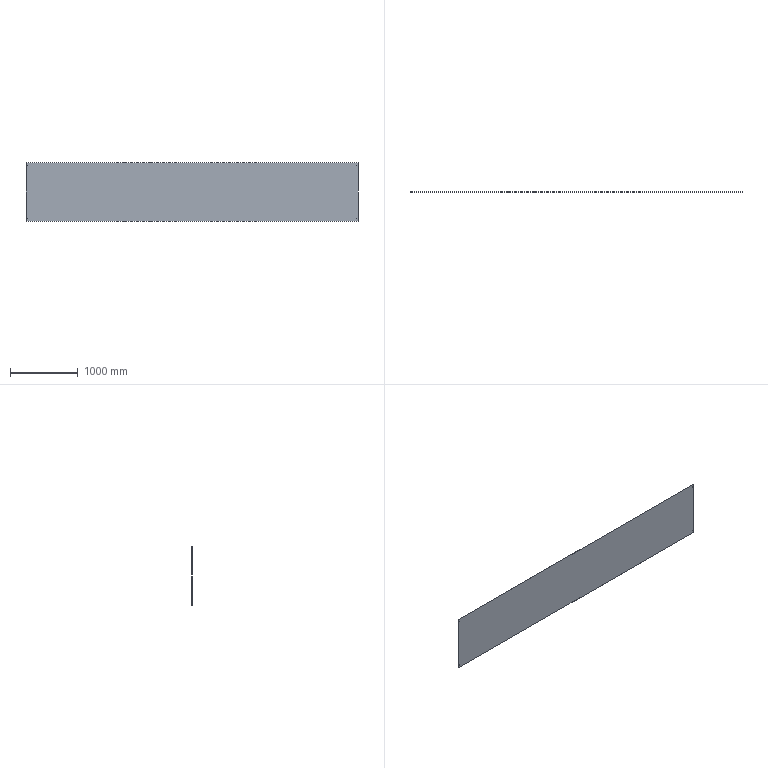Part | STEP file | 01-Cover plate | 1 solid | 14 faces | box 4900 x 0.6 x 870 mm | volume 2557612 mm3 | cylinder 8 | plane 6 | commonest cylinder face diameters 10 x8
STEP:
#1=CARTESIAN_POINT('',(0.,0.,0.));
#2=DIRECTION('',(0.,0.,1.));
#3=DIRECTION('',(1.,0.,0.));
#4=AXIS2_PLACEMENT_3D('',#1,#2,#3);
#5=CARTESIAN_POINT('',(4880.,0.,830.));
#6=VERTEX_POINT('',#5);
#7=CARTESIAN_POINT('',(4880.,0.6,830.));
#8=VERTEX_POINT('',#7);
#9=CARTESIAN_POINT('',(4880.,-19.4,830.));
#10=DIRECTION('',(0.,1.,0.));
#11=VECTOR('',#10,1.);
#12=LINE('',#9,#11);
#13=CARTESIAN_POINT('',(4880.,-19.4,825.));
#14=DIRECTION('',(0.,1.,0.));
#15=DIRECTION('',(0.,0.,1.));
#16=AXIS2_PLACEMENT_3D('',#13,#14,#15);
#17=CYLINDRICAL_SURFACE('',#16,5.);
#18=CARTESIAN_POINT('',(6.283,0.));
#19=DIRECTION('',(0.,1.));
#20=VECTOR('',#19,1.);
#21=LINE('',#18,#20);
#22=(GEOMETRIC_REPRESENTATION_CONTEXT(2)PARAMETRIC_REPRESENTATION_CONTEXT()REPRESENTATION_CONTEXT('',''));
#23=DEFINITIONAL_REPRESENTATION('',(#21),#22);
#24=PCURVE('',#17,#23);
#25=CARTESIAN_POINT('',(4880.,-19.4,825.));
#26=DIRECTION('',(0.,1.,0.));
#27=DIRECTION('',(0.,0.,1.));
#28=AXIS2_PLACEMENT_3D('',#25,#26,#27);
#29=CYLINDRICAL_SURFACE('',#28,5.);
#30=CARTESIAN_POINT('',(0.,0.));
#31=DIRECTION('',(0.,1.));
#32=VECTOR('',#31,1.);
#33=LINE('',#30,#32);
#34=(GEOMETRIC_REPRESENTATION_CONTEXT(2)PARAMETRIC_REPRESENTATION_CONTEXT()REPRESENTATION_CONTEXT('',''));
#35=DEFINITIONAL_REPRESENTATION('',(#33),#34);
#36=PCURVE('',#29,#35);
#37=SURFACE_CURVE('',#12,(#24,#36),.PCURVE_S1.);
#38=EDGE_CURVE('',#6,#8,#37,.T.);
#39=ORIENTED_EDGE('',*,*,#38,.T.);
#40=CARTESIAN_POINT('',(4880.,0.6,820.));
#41=VERTEX_POINT('',#40);
#42=CARTESIAN_POINT('',(4880.,0.6,825.));
#43=DIRECTION('',(0.,1.,0.));
#44=DIRECTION('',(0.,0.,1.));
#45=AXIS2_PLACEMENT_3D('',#42,#43,#44);
#46=CIRCLE('',#45,5.);
#47=CARTESIAN_POINT('',(0.,20.));
#48=DIRECTION('',(1.,0.));
#49=VECTOR('',#48,1.);
#50=LINE('',#47,#49);
#51=(GEOMETRIC_REPRESENTATION_CONTEXT(2)PARAMETRIC_REPRESENTATION_CONTEXT()REPRESENTATION_CONTEXT('',''));
#52=DEFINITIONAL_REPRESENTATION('',(#50),#51);
#53=PCURVE('',#17,#52);
#54=CARTESIAN_POINT('',(0.,0.6,0.));
#55=DIRECTION('',(0.,1.,0.));
#56=DIRECTION('',(0.,0.,1.));
#57=AXIS2_PLACEMENT_3D('',#54,#55,#56);
#58=PLANE('',#57);
#59=CARTESIAN_POINT('',(825.,4880.));
#60=DIRECTION('',(1.,0.));
#61=AXIS2_PLACEMENT_2D('',#59,#60);
#62=CIRCLE('',#61,5.);
#63=(GEOMETRIC_REPRESENTATION_CONTEXT(2)PARAMETRIC_REPRESENTATION_CONTEXT()REPRESENTATION_CONTEXT('',''));
#64=DEFINITIONAL_REPRESENTATION('',(#62),#63);
#65=PCURVE('',#58,#64);
#66=SURFACE_CURVE('',#46,(#53,#65),.PCURVE_S1.);
#67=EDGE_CURVE('',#41,#8,#66,.T.);
#68=ORIENTED_EDGE('',*,*,#67,.F.);
#69=CARTESIAN_POINT('',(4880.,0.,820.));
#70=VERTEX_POINT('',#69);
#71=CARTESIAN_POINT('',(4880.,-19.4,820.));
#72=DIRECTION('',(0.,1.,0.));
#73=VECTOR('',#72,1.);
#74=LINE('',#71,#73);
#75=CARTESIAN_POINT('',(3.142,0.));
#76=DIRECTION('',(0.,1.));
#77=VECTOR('',#76,1.);
#78=LINE('',#75,#77);
#79=(GEOMETRIC_REPRESENTATION_CONTEXT(2)PARAMETRIC_REPRESENTATION_CONTEXT()REPRESENTATION_CONTEXT('',''));
#80=DEFINITIONAL_REPRESENTATION('',(#78),#79);
#81=PCURVE('',#17,#80);
#82=CARTESIAN_POINT('',(3.142,0.));
#83=DIRECTION('',(0.,1.));
#84=VECTOR('',#83,1.);
#85=LINE('',#82,#84);
#86=(GEOMETRIC_REPRESENTATION_CONTEXT(2)PARAMETRIC_REPRESENTATION_CONTEXT()REPRESENTATION_CONTEXT('',''));
#87=DEFINITIONAL_REPRESENTATION('',(#85),#86);
#88=PCURVE('',#29,#87);
#89=SURFACE_CURVE('',#74,(#81,#88),.PCURVE_S1.);
#90=EDGE_CURVE('',#70,#41,#89,.T.);
#91=ORIENTED_EDGE('',*,*,#90,.F.);
#92=CARTESIAN_POINT('',(4880.,0.,825.));
#93=DIRECTION('',(0.,1.,0.));
#94=DIRECTION('',(0.,0.,1.));
#95=AXIS2_PLACEMENT_3D('',#92,#93,#94);
#96=CIRCLE('',#95,5.);
#97=CARTESIAN_POINT('',(0.,19.4));
#98=DIRECTION('',(1.,0.));
#99=VECTOR('',#98,1.);
#100=LINE('',#97,#99);
#101=(GEOMETRIC_REPRESENTATION_CONTEXT(2)PARAMETRIC_REPRESENTATION_CONTEXT()REPRESENTATION_CONTEXT('',''));
#102=DEFINITIONAL_REPRESENTATION('',(#100),#101);
#103=PCURVE('',#17,#102);
#104=CARTESIAN_POINT('',(0.,0.,0.));
#105=DIRECTION('',(0.,1.,0.));
#106=DIRECTION('',(0.,0.,1.));
#107=AXIS2_PLACEMENT_3D('',#104,#105,#106);
#108=PLANE('',#107);
#109=CARTESIAN_POINT('',(825.,4880.));
#110=DIRECTION('',(1.,0.));
#111=AXIS2_PLACEMENT_2D('',#109,#110);
#112=CIRCLE('',#111,5.);
#113=(GEOMETRIC_REPRESENTATION_CONTEXT(2)PARAMETRIC_REPRESENTATION_CONTEXT()REPRESENTATION_CONTEXT('',''));
#114=DEFINITIONAL_REPRESENTATION('',(#112),#113);
#115=PCURVE('',#108,#114);
#116=SURFACE_CURVE('',#96,(#103,#115),.PCURVE_S1.);
#117=EDGE_CURVE('',#70,#6,#116,.T.);
#118=ORIENTED_EDGE('',*,*,#117,.T.);
#119=EDGE_LOOP('',(#39,#68,#91,#118));
#120=FACE_BOUND('',#119,.F.);
#121=ADVANCED_FACE('',(#120),#17,.F.);
#122=CARTESIAN_POINT('',(4880.,0.,50.));
#123=VERTEX_POINT('',#122);
#124=CARTESIAN_POINT('',(4880.,0.6,50.));
#125=VERTEX_POINT('',#124);
#126=CARTESIAN_POINT('',(4880.,-19.4,50.));
#127=DIRECTION('',(0.,1.,0.));
#128=VECTOR('',#127,1.);
#129=LINE('',#126,#128);
#130=CARTESIAN_POINT('',(4880.,-19.4,45.));
#131=DIRECTION('',(0.,1.,0.));
#132=DIRECTION('',(0.,0.,1.));
#133=AXIS2_PLACEMENT_3D('',#130,#131,#132);
#134=CYLINDRICAL_SURFACE('',#133,5.);
#135=CARTESIAN_POINT('',(6.283,0.));
#136=DIRECTION('',(0.,1.));
#137=VECTOR('',#136,1.);
#138=LINE('',#135,#137);
#139=(GEOMETRIC_REPRESENTATION_CONTEXT(2)PARAMETRIC_REPRESENTATION_CONTEXT()REPRESENTATION_CONTEXT('',''));
#140=DEFINITIONAL_REPRESENTATION('',(#138),#139);
#141=PCURVE('',#134,#140);
#142=CARTESIAN_POINT('',(4880.,-19.4,45.));
#143=DIRECTION('',(0.,1.,0.));
#144=DIRECTION('',(0.,0.,1.));
#145=AXIS2_PLACEMENT_3D('',#142,#143,#144);
#146=CYLINDRICAL_SURFACE('',#145,5.);
#147=CARTESIAN_POINT('',(0.,0.));
#148=DIRECTION('',(0.,1.));
#149=VECTOR('',#148,1.);
#150=LINE('',#147,#149);
#151=(GEOMETRIC_REPRESENTATION_CONTEXT(2)PARAMETRIC_REPRESENTATION_CONTEXT()REPRESENTATION_CONTEXT('',''));
#152=DEFINITIONAL_REPRESENTATION('',(#150),#151);
#153=PCURVE('',#146,#152);
#154=SURFACE_CURVE('',#129,(#141,#153),.PCURVE_S1.);
#155=EDGE_CURVE('',#123,#125,#154,.T.);
#156=ORIENTED_EDGE('',*,*,#155,.T.);
#157=CARTESIAN_POINT('',(4880.,0.6,40.));
#158=VERTEX_POINT('',#157);
#159=CARTESIAN_POINT('',(4880.,0.6,45.));
#160=DIRECTION('',(0.,1.,0.));
#161=DIRECTION('',(0.,0.,1.));
#162=AXIS2_PLACEMENT_3D('',#159,#160,#161);
#163=CIRCLE('',#162,5.);
#164=CARTESIAN_POINT('',(0.,20.));
#165=DIRECTION('',(1.,0.));
#166=VECTOR('',#165,1.);
#167=LINE('',#164,#166);
#168=(GEOMETRIC_REPRESENTATION_CONTEXT(2)PARAMETRIC_REPRESENTATION_CONTEXT()REPRESENTATION_CONTEXT('',''));
#169=DEFINITIONAL_REPRESENTATION('',(#167),#168);
#170=PCURVE('',#134,#169);
#171=CARTESIAN_POINT('',(45.,4880.));
#172=DIRECTION('',(1.,0.));
#173=AXIS2_PLACEMENT_2D('',#171,#172);
#174=CIRCLE('',#173,5.);
#175=(GEOMETRIC_REPRESENTATION_CONTEXT(2)PARAMETRIC_REPRESENTATION_CONTEXT()REPRESENTATION_CONTEXT('',''));
#176=DEFINITIONAL_REPRESENTATION('',(#174),#175);
#177=PCURVE('',#58,#176);
#178=SURFACE_CURVE('',#163,(#170,#177),.PCURVE_S1.);
#179=EDGE_CURVE('',#158,#125,#178,.T.);
#180=ORIENTED_EDGE('',*,*,#179,.F.);
#181=CARTESIAN_POINT('',(4880.,0.,40.));
#182=VERTEX_POINT('',#181);
#183=CARTESIAN_POINT('',(4880.,-19.4,40.));
#184=DIRECTION('',(0.,1.,0.));
#185=VECTOR('',#184,1.);
#186=LINE('',#183,#185);
#187=CARTESIAN_POINT('',(3.142,0.));
#188=DIRECTION('',(0.,1.));
#189=VECTOR('',#188,1.);
#190=LINE('',#187,#189);
#191=(GEOMETRIC_REPRESENTATION_CONTEXT(2)PARAMETRIC_REPRESENTATION_CONTEXT()REPRESENTATION_CONTEXT('',''));
#192=DEFINITIONAL_REPRESENTATION('',(#190),#191);
#193=PCURVE('',#134,#192);
#194=CARTESIAN_POINT('',(3.142,0.));
#195=DIRECTION('',(0.,1.));
#196=VECTOR('',#195,1.);
#197=LINE('',#194,#196);
#198=(GEOMETRIC_REPRESENTATION_CONTEXT(2)PARAMETRIC_REPRESENTATION_CONTEXT()REPRESENTATION_CONTEXT('',''));
#199=DEFINITIONAL_REPRESENTATION('',(#197),#198);
#200=PCURVE('',#146,#199);
#201=SURFACE_CURVE('',#186,(#193,#200),.PCURVE_S1.);
#202=EDGE_CURVE('',#182,#158,#201,.T.);
#203=ORIENTED_EDGE('',*,*,#202,.F.);
#204=CARTESIAN_POINT('',(4880.,0.,45.));
#205=DIRECTION('',(0.,1.,0.));
#206=DIRECTION('',(0.,0.,1.));
#207=AXIS2_PLACEMENT_3D('',#204,#205,#206);
#208=CIRCLE('',#207,5.);
#209=CARTESIAN_POINT('',(0.,19.4));
#210=DIRECTION('',(1.,0.));
#211=VECTOR('',#210,1.);
#212=LINE('',#209,#211);
#213=(GEOMETRIC_REPRESENTATION_CONTEXT(2)PARAMETRIC_REPRESENTATION_CONTEXT()REPRESENTATION_CONTEXT('',''));
#214=DEFINITIONAL_REPRESENTATION('',(#212),#213);
#215=PCURVE('',#134,#214);
#216=CARTESIAN_POINT('',(45.,4880.));
#217=DIRECTION('',(1.,0.));
#218=AXIS2_PLACEMENT_2D('',#216,#217);
#219=CIRCLE('',#218,5.);
#220=(GEOMETRIC_REPRESENTATION_CONTEXT(2)PARAMETRIC_REPRESENTATION_CONTEXT()REPRESENTATION_CONTEXT('',''));
#221=DEFINITIONAL_REPRESENTATION('',(#219),#220);
#222=PCURVE('',#108,#221);
#223=SURFACE_CURVE('',#208,(#215,#222),.PCURVE_S1.);
#224=EDGE_CURVE('',#182,#123,#223,.T.);
#225=ORIENTED_EDGE('',*,*,#224,.T.);
#226=EDGE_LOOP('',(#156,#180,#203,#225));
#227=FACE_BOUND('',#226,.F.);
#228=ADVANCED_FACE('',(#227),#134,.F.);
#229=CARTESIAN_POINT('',(20.,0.,830.));
#230=VERTEX_POINT('',#229);
#231=CARTESIAN_POINT('',(20.,0.6,830.));
#232=VERTEX_POINT('',#231);
#233=CARTESIAN_POINT('',(20.,-19.4,830.));
#234=DIRECTION('',(0.,1.,0.));
#235=VECTOR('',#234,1.);
#236=LINE('',#233,#235);
#237=CARTESIAN_POINT('',(20.,-19.4,825.));
#238=DIRECTION('',(0.,1.,0.));
#239=DIRECTION('',(0.,0.,1.));
#240=AXIS2_PLACEMENT_3D('',#237,#238,#239);
#241=CYLINDRICAL_SURFACE('',#240,5.);
#242=CARTESIAN_POINT('',(6.283,0.));
#243=DIRECTION('',(0.,1.));
#244=VECTOR('',#243,1.);
#245=LINE('',#242,#244);
#246=(GEOMETRIC_REPRESENTATION_CONTEXT(2)PARAMETRIC_REPRESENTATION_CONTEXT()REPRESENTATION_CONTEXT('',''));
#247=DEFINITIONAL_REPRESENTATION('',(#245),#246);
#248=PCURVE('',#241,#247);
#249=CARTESIAN_POINT('',(20.,-19.4,825.));
#250=DIRECTION('',(0.,1.,0.));
#251=DIRECTION('',(0.,0.,1.));
#252=AXIS2_PLACEMENT_3D('',#249,#250,#251);
#253=CYLINDRICAL_SURFACE('',#252,5.);
#254=CARTESIAN_POINT('',(0.,0.));
#255=DIRECTION('',(0.,1.));
#256=VECTOR('',#255,1.);
#257=LINE('',#254,#256);
#258=(GEOMETRIC_REPRESENTATION_CONTEXT(2)PARAMETRIC_REPRESENTATION_CONTEXT()REPRESENTATION_CONTEXT('',''));
#259=DEFINITIONAL_REPRESENTATION('',(#257),#258);
#260=PCURVE('',#253,#259);
#261=SURFACE_CURVE('',#236,(#248,#260),.PCURVE_S1.);
#262=EDGE_CURVE('',#230,#232,#261,.T.);
#263=ORIENTED_EDGE('',*,*,#262,.T.);
#264=CARTESIAN_POINT('',(20.,0.6,820.));
#265=VERTEX_POINT('',#264);
#266=CARTESIAN_POINT('',(20.,0.6,825.));
#267=DIRECTION('',(0.,1.,0.));
#268=DIRECTION('',(0.,0.,1.));
#269=AXIS2_PLACEMENT_3D('',#266,#267,#268);
#270=CIRCLE('',#269,5.);
#271=CARTESIAN_POINT('',(0.,20.));
#272=DIRECTION('',(1.,0.));
#273=VECTOR('',#272,1.);
#274=LINE('',#271,#273);
#275=(GEOMETRIC_REPRESENTATION_CONTEXT(2)PARAMETRIC_REPRESENTATION_CONTEXT()REPRESENTATION_CONTEXT('',''));
#276=DEFINITIONAL_REPRESENTATION('',(#274),#275);
#277=PCURVE('',#241,#276);
#278=CARTESIAN_POINT('',(825.,20.));
#279=DIRECTION('',(1.,0.));
#280=AXIS2_PLACEMENT_2D('',#278,#279);
#281=CIRCLE('',#280,5.);
#282=(GEOMETRIC_REPRESENTATION_CONTEXT(2)PARAMETRIC_REPRESENTATION_CONTEXT()REPRESENTATION_CONTEXT('',''));
#283=DEFINITIONAL_REPRESENTATION('',(#281),#282);
#284=PCURVE('',#58,#283);
#285=SURFACE_CURVE('',#270,(#277,#284),.PCURVE_S1.);
#286=EDGE_CURVE('',#265,#232,#285,.T.);
#287=ORIENTED_EDGE('',*,*,#286,.F.);
#288=CARTESIAN_POINT('',(20.,0.,820.));
#289=VERTEX_POINT('',#288);
#290=CARTESIAN_POINT('',(20.,-19.4,820.));
#291=DIRECTION('',(0.,1.,0.));
#292=VECTOR('',#291,1.);
#293=LINE('',#290,#292);
#294=CARTESIAN_POINT('',(3.142,0.));
#295=DIRECTION('',(0.,1.));
#296=VECTOR('',#295,1.);
#297=LINE('',#294,#296);
#298=(GEOMETRIC_REPRESENTATION_CONTEXT(2)PARAMETRIC_REPRESENTATION_CONTEXT()REPRESENTATION_CONTEXT('',''));
#299=DEFINITIONAL_REPRESENTATION('',(#297),#298);
#300=PCURVE('',#241,#299);
#301=CARTESIAN_POINT('',(3.142,0.));
#302=DIRECTION('',(0.,1.));
#303=VECTOR('',#302,1.);
#304=LINE('',#301,#303);
#305=(GEOMETRIC_REPRESENTATION_CONTEXT(2)PARAMETRIC_REPRESENTATION_CONTEXT()REPRESENTATION_CONTEXT('',''));
#306=DEFINITIONAL_REPRESENTATION('',(#304),#305);
#307=PCURVE('',#253,#306);
#308=SURFACE_CURVE('',#293,(#300,#307),.PCURVE_S1.);
#309=EDGE_CURVE('',#289,#265,#308,.T.);
#310=ORIENTED_EDGE('',*,*,#309,.F.);
#311=CARTESIAN_POINT('',(20.,0.,825.));
#312=DIRECTION('',(0.,1.,0.));
#313=DIRECTION('',(0.,0.,1.));
#314=AXIS2_PLACEMENT_3D('',#311,#312,#313);
#315=CIRCLE('',#314,5.);
#316=CARTESIAN_POINT('',(0.,19.4));
#317=DIRECTION('',(1.,0.));
#318=VECTOR('',#317,1.);
#319=LINE('',#316,#318);
#320=(GEOMETRIC_REPRESENTATION_CONTEXT(2)PARAMETRIC_REPRESENTATION_CONTEXT()REPRESENTATION_CONTEXT('',''));
#321=DEFINITIONAL_REPRESENTATION('',(#319),#320);
#322=PCURVE('',#241,#321);
#323=CARTESIAN_POINT('',(825.,20.));
#324=DIRECTION('',(1.,0.));
#325=AXIS2_PLACEMENT_2D('',#323,#324);
#326=CIRCLE('',#325,5.);
#327=(GEOMETRIC_REPRESENTATION_CONTEXT(2)PARAMETRIC_REPRESENTATION_CONTEXT()REPRESENTATION_CONTEXT('',''));
#328=DEFINITIONAL_REPRESENTATION('',(#326),#327);
#329=PCURVE('',#108,#328);
#330=SURFACE_CURVE('',#315,(#322,#329),.PCURVE_S1.);
#331=EDGE_CURVE('',#289,#230,#330,.T.);
#332=ORIENTED_EDGE('',*,*,#331,.T.);
#333=EDGE_LOOP('',(#263,#287,#310,#332));
#334=FACE_BOUND('',#333,.F.);
#335=ADVANCED_FACE('',(#334),#241,.F.);
#336=CARTESIAN_POINT('',(20.,0.,50.));
#337=VERTEX_POINT('',#336);
#338=CARTESIAN_POINT('',(20.,0.6,50.));
#339=VERTEX_POINT('',#338);
#340=CARTESIAN_POINT('',(20.,-19.4,50.));
#341=DIRECTION('',(0.,1.,0.));
#342=VECTOR('',#341,1.);
#343=LINE('',#340,#342);
#344=CARTESIAN_POINT('',(20.,-19.4,45.));
#345=DIRECTION('',(0.,1.,0.));
#346=DIRECTION('',(0.,0.,1.));
#347=AXIS2_PLACEMENT_3D('',#344,#345,#346);
#348=CYLINDRICAL_SURFACE('',#347,5.);
#349=CARTESIAN_POINT('',(6.283,0.));
#350=DIRECTION('',(0.,1.));
#351=VECTOR('',#350,1.);
#352=LINE('',#349,#351);
#353=(GEOMETRIC_REPRESENTATION_CONTEXT(2)PARAMETRIC_REPRESENTATION_CONTEXT()REPRESENTATION_CONTEXT('',''));
#354=DEFINITIONAL_REPRESENTATION('',(#352),#353);
#355=PCURVE('',#348,#354);
#356=CARTESIAN_POINT('',(20.,-19.4,45.));
#357=DIRECTION('',(0.,1.,0.));
#358=DIRECTION('',(0.,0.,1.));
#359=AXIS2_PLACEMENT_3D('',#356,#357,#358);
#360=CYLINDRICAL_SURFACE('',#359,5.);
#361=CARTESIAN_POINT('',(0.,0.));
#362=DIRECTION('',(0.,1.));
#363=VECTOR('',#362,1.);
#364=LINE('',#361,#363);
#365=(GEOMETRIC_REPRESENTATION_CONTEXT(2)PARAMETRIC_REPRESENTATION_CONTEXT()REPRESENTATION_CONTEXT('',''));
#366=DEFINITIONAL_REPRESENTATION('',(#364),#365);
#367=PCURVE('',#360,#366);
#368=SURFACE_CURVE('',#343,(#355,#367),.PCURVE_S1.);
#369=EDGE_CURVE('',#337,#339,#368,.T.);
#370=ORIENTED_EDGE('',*,*,#369,.T.);
#371=CARTESIAN_POINT('',(20.,0.6,40.));
#372=VERTEX_POINT('',#371);
#373=CARTESIAN_POINT('',(20.,0.6,45.));
#374=DIRECTION('',(0.,1.,0.));
#375=DIRECTION('',(0.,0.,1.));
#376=AXIS2_PLACEMENT_3D('',#373,#374,#375);
#377=CIRCLE('',#376,5.);
#378=CARTESIAN_POINT('',(0.,20.));
#379=DIRECTION('',(1.,0.));
#380=VECTOR('',#379,1.);
#381=LINE('',#378,#380);
#382=(GEOMETRIC_REPRESENTATION_CONTEXT(2)PARAMETRIC_REPRESENTATION_CONTEXT()REPRESENTATION_CONTEXT('',''));
#383=DEFINITIONAL_REPRESENTATION('',(#381),#382);
#384=PCURVE('',#348,#383);
#385=CARTESIAN_POINT('',(45.,20.));
#386=DIRECTION('',(1.,0.));
#387=AXIS2_PLACEMENT_2D('',#385,#386);
#388=CIRCLE('',#387,5.);
#389=(GEOMETRIC_REPRESENTATION_CONTEXT(2)PARAMETRIC_REPRESENTATION_CONTEXT()REPRESENTATION_CONTEXT('',''));
#390=DEFINITIONAL_REPRESENTATION('',(#388),#389);
#391=PCURVE('',#58,#390);
#392=SURFACE_CURVE('',#377,(#384,#391),.PCURVE_S1.);
#393=EDGE_CURVE('',#372,#339,#392,.T.);
#394=ORIENTED_EDGE('',*,*,#393,.F.);
#395=CARTESIAN_POINT('',(20.,0.,40.));
#396=VERTEX_POINT('',#395);
#397=CARTESIAN_POINT('',(20.,-19.4,40.));
#398=DIRECTION('',(0.,1.,0.));
#399=VECTOR('',#398,1.);
#400=LINE('',#397,#399);
#401=CARTESIAN_POINT('',(3.142,0.));
#402=DIRECTION('',(0.,1.));
#403=VECTOR('',#402,1.);
#404=LINE('',#401,#403);
#405=(GEOMETRIC_REPRESENTATION_CONTEXT(2)PARAMETRIC_REPRESENTATION_CONTEXT()REPRESENTATION_CONTEXT('',''));
#406=DEFINITIONAL_REPRESENTATION('',(#404),#405);
#407=PCURVE('',#348,#406);
#408=CARTESIAN_POINT('',(3.142,0.));
#409=DIRECTION('',(0.,1.));
#410=VECTOR('',#409,1.);
#411=LINE('',#408,#410);
#412=(GEOMETRIC_REPRESENTATION_CONTEXT(2)PARAMETRIC_REPRESENTATION_CONTEXT()REPRESENTATION_CONTEXT('',''));
#413=DEFINITIONAL_REPRESENTATION('',(#411),#412);
#414=PCURVE('',#360,#413);
#415=SURFACE_CURVE('',#400,(#407,#414),.PCURVE_S1.);
#416=EDGE_CURVE('',#396,#372,#415,.T.);
#417=ORIENTED_EDGE('',*,*,#416,.F.);
#418=CARTESIAN_POINT('',(20.,0.,45.));
#419=DIRECTION('',(0.,1.,0.));
#420=DIRECTION('',(0.,0.,1.));
#421=AXIS2_PLACEMENT_3D('',#418,#419,#420);
#422=CIRCLE('',#421,5.);
#423=CARTESIAN_POINT('',(0.,19.4));
#424=DIRECTION('',(1.,0.));
#425=VECTOR('',#424,1.);
#426=LINE('',#423,#425);
#427=(GEOMETRIC_REPRESENTATION_CONTEXT(2)PARAMETRIC_REPRESENTATION_CONTEXT()REPRESENTATION_CONTEXT('',''));
#428=DEFINITIONAL_REPRESENTATION('',(#426),#427);
#429=PCURVE('',#348,#428);
#430=CARTESIAN_POINT('',(45.,20.));
#431=DIRECTION('',(1.,0.));
#432=AXIS2_PLACEMENT_2D('',#430,#431);
#433=CIRCLE('',#432,5.);
#434=(GEOMETRIC_REPRESENTATION_CONTEXT(2)PARAMETRIC_REPRESENTATION_CONTEXT()REPRESENTATION_CONTEXT('',''));
#435=DEFINITIONAL_REPRESENTATION('',(#433),#434);
#436=PCURVE('',#108,#435);
#437=SURFACE_CURVE('',#422,(#429,#436),.PCURVE_S1.);
#438=EDGE_CURVE('',#396,#337,#437,.T.);
#439=ORIENTED_EDGE('',*,*,#438,.T.);
#440=EDGE_LOOP('',(#370,#394,#417,#439));
#441=FACE_BOUND('',#440,.F.);
#442=ADVANCED_FACE('',(#441),#348,.F.);
#443=CARTESIAN_POINT('',(0.,0.,0.));
#444=VERTEX_POINT('',#443);
#445=CARTESIAN_POINT('',(0.,0.,870.));
#446=VERTEX_POINT('',#445);
#447=CARTESIAN_POINT('',(0.,0.,0.));
#448=DIRECTION('',(0.,0.,1.));
#449=VECTOR('',#448,1.);
#450=LINE('',#447,#449);
#451=CARTESIAN_POINT('',(0.,0.6,0.));
#452=DIRECTION('',(1.,0.,0.));
#453=DIRECTION('',(0.,0.,-1.));
#454=AXIS2_PLACEMENT_3D('',#451,#452,#453);
#455=PLANE('',#454);
#456=CARTESIAN_POINT('',(0.,-0.6));
#457=DIRECTION('',(-1.,0.));
#458=VECTOR('',#457,1.);
#459=LINE('',#456,#458);
#460=(GEOMETRIC_REPRESENTATION_CONTEXT(2)PARAMETRIC_REPRESENTATION_CONTEXT()REPRESENTATION_CONTEXT('',''));
#461=DEFINITIONAL_REPRESENTATION('',(#459),#460);
#462=PCURVE('',#455,#461);
#463=CARTESIAN_POINT('',(0.,0.));
#464=DIRECTION('',(1.,0.));
#465=VECTOR('',#464,1.);
#466=LINE('',#463,#465);
#467=(GEOMETRIC_REPRESENTATION_CONTEXT(2)PARAMETRIC_REPRESENTATION_CONTEXT()REPRESENTATION_CONTEXT('',''));
#468=DEFINITIONAL_REPRESENTATION('',(#466),#467);
#469=PCURVE('',#108,#468);
#470=SURFACE_CURVE('',#450,(#462,#469),.PCURVE_S1.);
#471=EDGE_CURVE('',#444,#446,#470,.T.);
#472=ORIENTED_EDGE('',*,*,#471,.T.);
#473=CARTESIAN_POINT('',(0.,0.6,870.));
#474=VERTEX_POINT('',#473);
#475=CARTESIAN_POINT('',(0.,0.6,870.));
#476=DIRECTION('',(0.,-1.,0.));
#477=VECTOR('',#476,1.);
#478=LINE('',#475,#477);
#479=CARTESIAN_POINT('',(-870.,0.));
#480=DIRECTION('',(0.,-1.));
#481=VECTOR('',#480,1.);
#482=LINE('',#479,#481);
#483=(GEOMETRIC_REPRESENTATION_CONTEXT(2)PARAMETRIC_REPRESENTATION_CONTEXT()REPRESENTATION_CONTEXT('',''));
#484=DEFINITIONAL_REPRESENTATION('',(#482),#483);
#485=PCURVE('',#455,#484);
#486=CARTESIAN_POINT('',(0.,0.6,870.));
#487=DIRECTION('',(0.,0.,-1.));
#488=DIRECTION('',(-1.,0.,0.));
#489=AXIS2_PLACEMENT_3D('',#486,#487,#488);
#490=PLANE('',#489);
#491=CARTESIAN_POINT('',(0.,0.));
#492=DIRECTION('',(0.,-1.));
#493=VECTOR('',#492,1.);
#494=LINE('',#491,#493);
#495=(GEOMETRIC_REPRESENTATION_CONTEXT(2)PARAMETRIC_REPRESENTATION_CONTEXT()REPRESENTATION_CONTEXT('',''));
#496=DEFINITIONAL_REPRESENTATION('',(#494),#495);
#497=PCURVE('',#490,#496);
#498=SURFACE_CURVE('',#478,(#485,#497),.PCURVE_S1.);
#499=EDGE_CURVE('',#474,#446,#498,.T.);
#500=ORIENTED_EDGE('',*,*,#499,.F.);
#501=CARTESIAN_POINT('',(0.,0.6,0.));
#502=VERTEX_POINT('',#501);
#503=CARTESIAN_POINT('',(0.,0.6,0.));
#504=DIRECTION('',(0.,0.,1.));
#505=VECTOR('',#504,1.);
#506=LINE('',#503,#505);
#507=CARTESIAN_POINT('',(0.,0.));
#508=DIRECTION('',(-1.,0.));
#509=VECTOR('',#508,1.);
#510=LINE('',#507,#509);
#511=(GEOMETRIC_REPRESENTATION_CONTEXT(2)PARAMETRIC_REPRESENTATION_CONTEXT()REPRESENTATION_CONTEXT('',''));
#512=DEFINITIONAL_REPRESENTATION('',(#510),#511);
#513=PCURVE('',#455,#512);
#514=CARTESIAN_POINT('',(0.,0.));
#515=DIRECTION('',(1.,0.));
#516=VECTOR('',#515,1.);
#517=LINE('',#514,#516);
#518=(GEOMETRIC_REPRESENTATION_CONTEXT(2)PARAMETRIC_REPRESENTATION_CONTEXT()REPRESENTATION_CONTEXT('',''));
#519=DEFINITIONAL_REPRESENTATION('',(#517),#518);
#520=PCURVE('',#58,#519);
#521=SURFACE_CURVE('',#506,(#513,#520),.PCURVE_S1.);
#522=EDGE_CURVE('',#502,#474,#521,.T.);
#523=ORIENTED_EDGE('',*,*,#522,.F.);
#524=CARTESIAN_POINT('',(0.,0.6,0.));
#525=DIRECTION('',(0.,-1.,0.));
#526=VECTOR('',#525,1.);
#527=LINE('',#524,#526);
#528=CARTESIAN_POINT('',(0.,0.));
#529=DIRECTION('',(0.,-1.));
#530=VECTOR('',#529,1.);
#531=LINE('',#528,#530);
#532=(GEOMETRIC_REPRESENTATION_CONTEXT(2)PARAMETRIC_REPRESENTATION_CONTEXT()REPRESENTATION_CONTEXT('',''));
#533=DEFINITIONAL_REPRESENTATION('',(#531),#532);
#534=PCURVE('',#455,#533);
#535=CARTESIAN_POINT('',(0.,0.6,0.));
#536=DIRECTION('',(0.,0.,1.));
#537=DIRECTION('',(1.,0.,0.));
#538=AXIS2_PLACEMENT_3D('',#535,#536,#537);
#539=PLANE('',#538);
#540=CARTESIAN_POINT('',(0.,0.));
#541=DIRECTION('',(0.,-1.));
#542=VECTOR('',#541,1.);
#543=LINE('',#540,#542);
#544=(GEOMETRIC_REPRESENTATION_CONTEXT(2)PARAMETRIC_REPRESENTATION_CONTEXT()REPRESENTATION_CONTEXT('',''));
#545=DEFINITIONAL_REPRESENTATION('',(#543),#544);
#546=PCURVE('',#539,#545);
#547=SURFACE_CURVE('',#527,(#534,#546),.PCURVE_S1.);
#548=EDGE_CURVE('',#502,#444,#547,.T.);
#549=ORIENTED_EDGE('',*,*,#548,.T.);
#550=EDGE_LOOP('',(#472,#500,#523,#549));
#551=FACE_BOUND('',#550,.T.);
#552=ADVANCED_FACE('',(#551),#455,.F.);
#553=CARTESIAN_POINT('',(4900.,0.,870.));
#554=VERTEX_POINT('',#553);
#555=CARTESIAN_POINT('',(0.,0.,870.));
#556=DIRECTION('',(1.,0.,0.));
#557=VECTOR('',#556,1.);
#558=LINE('',#555,#557);
#559=CARTESIAN_POINT('',(0.,-0.6));
#560=DIRECTION('',(-1.,0.));
#561=VECTOR('',#560,1.);
#562=LINE('',#559,#561);
#563=(GEOMETRIC_REPRESENTATION_CONTEXT(2)PARAMETRIC_REPRESENTATION_CONTEXT()REPRESENTATION_CONTEXT('',''));
#564=DEFINITIONAL_REPRESENTATION('',(#562),#563);
#565=PCURVE('',#490,#564);
#566=CARTESIAN_POINT('',(870.,0.));
#567=DIRECTION('',(0.,1.));
#568=VECTOR('',#567,1.);
#569=LINE('',#566,#568);
#570=(GEOMETRIC_REPRESENTATION_CONTEXT(2)PARAMETRIC_REPRESENTATION_CONTEXT()REPRESENTATION_CONTEXT('',''));
#571=DEFINITIONAL_REPRESENTATION('',(#569),#570);
#572=PCURVE('',#108,#571);
#573=SURFACE_CURVE('',#558,(#565,#572),.PCURVE_S1.);
#574=EDGE_CURVE('',#446,#554,#573,.T.);
#575=ORIENTED_EDGE('',*,*,#574,.T.);
#576=CARTESIAN_POINT('',(4900.,0.6,870.));
#577=VERTEX_POINT('',#576);
#578=CARTESIAN_POINT('',(4900.,0.6,870.));
#579=DIRECTION('',(0.,-1.,0.));
#580=VECTOR('',#579,1.);
#581=LINE('',#578,#580);
#582=CARTESIAN_POINT('',(-4900.,0.));
#583=DIRECTION('',(0.,-1.));
#584=VECTOR('',#583,1.);
#585=LINE('',#582,#584);
#586=(GEOMETRIC_REPRESENTATION_CONTEXT(2)PARAMETRIC_REPRESENTATION_CONTEXT()REPRESENTATION_CONTEXT('',''));
#587=DEFINITIONAL_REPRESENTATION('',(#585),#586);
#588=PCURVE('',#490,#587);
#589=CARTESIAN_POINT('',(4900.,0.6,0.));
#590=DIRECTION('',(-1.,0.,0.));
#591=DIRECTION('',(0.,0.,1.));
#592=AXIS2_PLACEMENT_3D('',#589,#590,#591);
#593=PLANE('',#592);
#594=CARTESIAN_POINT('',(870.,0.));
#595=DIRECTION('',(0.,-1.));
#596=VECTOR('',#595,1.);
#597=LINE('',#594,#596);
#598=(GEOMETRIC_REPRESENTATION_CONTEXT(2)PARAMETRIC_REPRESENTATION_CONTEXT()REPRESENTATION_CONTEXT('',''));
#599=DEFINITIONAL_REPRESENTATION('',(#597),#598);
#600=PCURVE('',#593,#599);
#601=SURFACE_CURVE('',#581,(#588,#600),.PCURVE_S1.);
#602=EDGE_CURVE('',#577,#554,#601,.T.);
#603=ORIENTED_EDGE('',*,*,#602,.F.);
#604=CARTESIAN_POINT('',(0.,0.6,870.));
#605=DIRECTION('',(1.,0.,0.));
#606=VECTOR('',#605,1.);
#607=LINE('',#604,#606);
#608=CARTESIAN_POINT('',(0.,0.));
#609=DIRECTION('',(-1.,0.));
#610=VECTOR('',#609,1.);
#611=LINE('',#608,#610);
#612=(GEOMETRIC_REPRESENTATION_CONTEXT(2)PARAMETRIC_REPRESENTATION_CONTEXT()REPRESENTATION_CONTEXT('',''));
#613=DEFINITIONAL_REPRESENTATION('',(#611),#612);
#614=PCURVE('',#490,#613);
#615=CARTESIAN_POINT('',(870.,0.));
#616=DIRECTION('',(0.,1.));
#617=VECTOR('',#616,1.);
#618=LINE('',#615,#617);
#619=(GEOMETRIC_REPRESENTATION_CONTEXT(2)PARAMETRIC_REPRESENTATION_CONTEXT()REPRESENTATION_CONTEXT('',''));
#620=DEFINITIONAL_REPRESENTATION('',(#618),#619);
#621=PCURVE('',#58,#620);
#622=SURFACE_CURVE('',#607,(#614,#621),.PCURVE_S1.);
#623=EDGE_CURVE('',#474,#577,#622,.T.);
#624=ORIENTED_EDGE('',*,*,#623,.F.);
#625=ORIENTED_EDGE('',*,*,#499,.T.);
#626=EDGE_LOOP('',(#575,#603,#624,#625));
#627=FACE_BOUND('',#626,.T.);
#628=ADVANCED_FACE('',(#627),#490,.F.);
#629=CARTESIAN_POINT('',(4900.,0.,0.));
#630=VERTEX_POINT('',#629);
#631=CARTESIAN_POINT('',(4900.,0.,0.));
#632=DIRECTION('',(0.,0.,-1.));
#633=VECTOR('',#632,1.);
#634=LINE('',#631,#633);
#635=CARTESIAN_POINT('',(0.,-0.6));
#636=DIRECTION('',(-1.,0.));
#637=VECTOR('',#636,1.);
#638=LINE('',#635,#637);
#639=(GEOMETRIC_REPRESENTATION_CONTEXT(2)PARAMETRIC_REPRESENTATION_CONTEXT()REPRESENTATION_CONTEXT('',''));
#640=DEFINITIONAL_REPRESENTATION('',(#638),#639);
#641=PCURVE('',#593,#640);
#642=CARTESIAN_POINT('',(0.,4900.));
#643=DIRECTION('',(-1.,0.));
#644=VECTOR('',#643,1.);
#645=LINE('',#642,#644);
#646=(GEOMETRIC_REPRESENTATION_CONTEXT(2)PARAMETRIC_REPRESENTATION_CONTEXT()REPRESENTATION_CONTEXT('',''));
#647=DEFINITIONAL_REPRESENTATION('',(#645),#646);
#648=PCURVE('',#108,#647);
#649=SURFACE_CURVE('',#634,(#641,#648),.PCURVE_S1.);
#650=EDGE_CURVE('',#554,#630,#649,.T.);
#651=ORIENTED_EDGE('',*,*,#650,.T.);
#652=CARTESIAN_POINT('',(4900.,0.6,0.));
#653=VERTEX_POINT('',#652);
#654=CARTESIAN_POINT('',(4900.,0.6,0.));
#655=DIRECTION('',(0.,-1.,0.));
#656=VECTOR('',#655,1.);
#657=LINE('',#654,#656);
#658=CARTESIAN_POINT('',(0.,0.));
#659=DIRECTION('',(0.,-1.));
#660=VECTOR('',#659,1.);
#661=LINE('',#658,#660);
#662=(GEOMETRIC_REPRESENTATION_CONTEXT(2)PARAMETRIC_REPRESENTATION_CONTEXT()REPRESENTATION_CONTEXT('',''));
#663=DEFINITIONAL_REPRESENTATION('',(#661),#662);
#664=PCURVE('',#593,#663);
#665=CARTESIAN_POINT('',(4900.,0.));
#666=DIRECTION('',(0.,-1.));
#667=VECTOR('',#666,1.);
#668=LINE('',#665,#667);
#669=(GEOMETRIC_REPRESENTATION_CONTEXT(2)PARAMETRIC_REPRESENTATION_CONTEXT()REPRESENTATION_CONTEXT('',''));
#670=DEFINITIONAL_REPRESENTATION('',(#668),#669);
#671=PCURVE('',#539,#670);
#672=SURFACE_CURVE('',#657,(#664,#671),.PCURVE_S1.);
#673=EDGE_CURVE('',#653,#630,#672,.T.);
#674=ORIENTED_EDGE('',*,*,#673,.F.);
#675=CARTESIAN_POINT('',(4900.,0.6,0.));
#676=DIRECTION('',(0.,0.,-1.));
#677=VECTOR('',#676,1.);
#678=LINE('',#675,#677);
#679=CARTESIAN_POINT('',(0.,0.));
#680=DIRECTION('',(-1.,0.));
#681=VECTOR('',#680,1.);
#682=LINE('',#679,#681);
#683=(GEOMETRIC_REPRESENTATION_CONTEXT(2)PARAMETRIC_REPRESENTATION_CONTEXT()REPRESENTATION_CONTEXT('',''));
#684=DEFINITIONAL_REPRESENTATION('',(#682),#683);
#685=PCURVE('',#593,#684);
#686=CARTESIAN_POINT('',(0.,4900.));
#687=DIRECTION('',(-1.,0.));
#688=VECTOR('',#687,1.);
#689=LINE('',#686,#688);
#690=(GEOMETRIC_REPRESENTATION_CONTEXT(2)PARAMETRIC_REPRESENTATION_CONTEXT()REPRESENTATION_CONTEXT('',''));
#691=DEFINITIONAL_REPRESENTATION('',(#689),#690);
#692=PCURVE('',#58,#691);
#693=SURFACE_CURVE('',#678,(#685,#692),.PCURVE_S1.);
#694=EDGE_CURVE('',#577,#653,#693,.T.);
#695=ORIENTED_EDGE('',*,*,#694,.F.);
#696=ORIENTED_EDGE('',*,*,#602,.T.);
#697=EDGE_LOOP('',(#651,#674,#695,#696));
#698=FACE_BOUND('',#697,.T.);
#699=ADVANCED_FACE('',(#698),#593,.F.);
#700=CARTESIAN_POINT('',(0.,0.,0.));
#701=DIRECTION('',(-1.,0.,0.));
#702=VECTOR('',#701,1.);
#703=LINE('',#700,#702);
#704=CARTESIAN_POINT('',(0.,-0.6));
#705=DIRECTION('',(-1.,0.));
#706=VECTOR('',#705,1.);
#707=LINE('',#704,#706);
#708=(GEOMETRIC_REPRESENTATION_CONTEXT(2)PARAMETRIC_REPRESENTATION_CONTEXT()REPRESENTATION_CONTEXT('',''));
#709=DEFINITIONAL_REPRESENTATION('',(#707),#708);
#710=PCURVE('',#539,#709);
#711=CARTESIAN_POINT('',(0.,0.));
#712=DIRECTION('',(0.,-1.));
#713=VECTOR('',#712,1.);
#714=LINE('',#711,#713);
#715=(GEOMETRIC_REPRESENTATION_CONTEXT(2)PARAMETRIC_REPRESENTATION_CONTEXT()REPRESENTATION_CONTEXT('',''));
#716=DEFINITIONAL_REPRESENTATION('',(#714),#715);
#717=PCURVE('',#108,#716);
#718=SURFACE_CURVE('',#703,(#710,#717),.PCURVE_S1.);
#719=EDGE_CURVE('',#630,#444,#718,.T.);
#720=ORIENTED_EDGE('',*,*,#719,.T.);
#721=ORIENTED_EDGE('',*,*,#548,.F.);
#722=CARTESIAN_POINT('',(0.,0.6,0.));
#723=DIRECTION('',(-1.,0.,0.));
#724=VECTOR('',#723,1.);
#725=LINE('',#722,#724);
#726=CARTESIAN_POINT('',(0.,0.));
#727=DIRECTION('',(-1.,0.));
#728=VECTOR('',#727,1.);
#729=LINE('',#726,#728);
#730=(GEOMETRIC_REPRESENTATION_CONTEXT(2)PARAMETRIC_REPRESENTATION_CONTEXT()REPRESENTATION_CONTEXT('',''));
#731=DEFINITIONAL_REPRESENTATION('',(#729),#730);
#732=PCURVE('',#539,#731);
#733=CARTESIAN_POINT('',(0.,0.));
#734=DIRECTION('',(0.,-1.));
#735=VECTOR('',#734,1.);
#736=LINE('',#733,#735);
#737=(GEOMETRIC_REPRESENTATION_CONTEXT(2)PARAMETRIC_REPRESENTATION_CONTEXT()REPRESENTATION_CONTEXT('',''));
#738=DEFINITIONAL_REPRESENTATION('',(#736),#737);
#739=PCURVE('',#58,#738);
#740=SURFACE_CURVE('',#725,(#732,#739),.PCURVE_S1.);
#741=EDGE_CURVE('',#653,#502,#740,.T.);
#742=ORIENTED_EDGE('',*,*,#741,.F.);
#743=ORIENTED_EDGE('',*,*,#673,.T.);
#744=EDGE_LOOP('',(#720,#721,#742,#743));
#745=FACE_BOUND('',#744,.T.);
#746=ADVANCED_FACE('',(#745),#539,.F.);
#747=CARTESIAN_POINT('',(4880.,0.6,825.));
#748=DIRECTION('',(0.,1.,0.));
#749=DIRECTION('',(0.,0.,1.));
#750=AXIS2_PLACEMENT_3D('',#747,#748,#749);
#751=CIRCLE('',#750,5.);
#752=CARTESIAN_POINT('',(825.,4880.));
#753=DIRECTION('',(1.,0.));
#754=AXIS2_PLACEMENT_2D('',#752,#753);
#755=CIRCLE('',#754,5.);
#756=(GEOMETRIC_REPRESENTATION_CONTEXT(2)PARAMETRIC_REPRESENTATION_CONTEXT()REPRESENTATION_CONTEXT('',''));
#757=DEFINITIONAL_REPRESENTATION('',(#755),#756);
#758=PCURVE('',#58,#757);
#759=CARTESIAN_POINT('',(0.,20.));
#760=DIRECTION('',(1.,0.));
#761=VECTOR('',#760,1.);
#762=LINE('',#759,#761);
#763=(GEOMETRIC_REPRESENTATION_CONTEXT(2)PARAMETRIC_REPRESENTATION_CONTEXT()REPRESENTATION_CONTEXT('',''));
#764=DEFINITIONAL_REPRESENTATION('',(#762),#763);
#765=PCURVE('',#29,#764);
#766=SURFACE_CURVE('',#751,(#758,#765),.PCURVE_S1.);
#767=EDGE_CURVE('',#8,#41,#766,.T.);
#768=ORIENTED_EDGE('',*,*,#767,.F.);
#769=ORIENTED_EDGE('',*,*,#67,.F.);
#770=EDGE_LOOP('',(#768,#769));
#771=FACE_BOUND('',#770,.T.);
#772=CARTESIAN_POINT('',(4880.,0.6,45.));
#773=DIRECTION('',(0.,1.,0.));
#774=DIRECTION('',(0.,0.,1.));
#775=AXIS2_PLACEMENT_3D('',#772,#773,#774);
#776=CIRCLE('',#775,5.);
#777=CARTESIAN_POINT('',(45.,4880.));
#778=DIRECTION('',(1.,0.));
#779=AXIS2_PLACEMENT_2D('',#777,#778);
#780=CIRCLE('',#779,5.);
#781=(GEOMETRIC_REPRESENTATION_CONTEXT(2)PARAMETRIC_REPRESENTATION_CONTEXT()REPRESENTATION_CONTEXT('',''));
#782=DEFINITIONAL_REPRESENTATION('',(#780),#781);
#783=PCURVE('',#58,#782);
#784=CARTESIAN_POINT('',(0.,20.));
#785=DIRECTION('',(1.,0.));
#786=VECTOR('',#785,1.);
#787=LINE('',#784,#786);
#788=(GEOMETRIC_REPRESENTATION_CONTEXT(2)PARAMETRIC_REPRESENTATION_CONTEXT()REPRESENTATION_CONTEXT('',''));
#789=DEFINITIONAL_REPRESENTATION('',(#787),#788);
#790=PCURVE('',#146,#789);
#791=SURFACE_CURVE('',#776,(#783,#790),.PCURVE_S1.);
#792=EDGE_CURVE('',#125,#158,#791,.T.);
#793=ORIENTED_EDGE('',*,*,#792,.F.);
#794=ORIENTED_EDGE('',*,*,#179,.F.);
#795=EDGE_LOOP('',(#793,#794));
#796=FACE_BOUND('',#795,.T.);
#797=CARTESIAN_POINT('',(20.,0.6,825.));
#798=DIRECTION('',(0.,1.,0.));
#799=DIRECTION('',(0.,0.,1.));
#800=AXIS2_PLACEMENT_3D('',#797,#798,#799);
#801=CIRCLE('',#800,5.);
#802=CARTESIAN_POINT('',(825.,20.));
#803=DIRECTION('',(1.,0.));
#804=AXIS2_PLACEMENT_2D('',#802,#803);
#805=CIRCLE('',#804,5.);
#806=(GEOMETRIC_REPRESENTATION_CONTEXT(2)PARAMETRIC_REPRESENTATION_CONTEXT()REPRESENTATION_CONTEXT('',''));
#807=DEFINITIONAL_REPRESENTATION('',(#805),#806);
#808=PCURVE('',#58,#807);
#809=CARTESIAN_POINT('',(0.,20.));
#810=DIRECTION('',(1.,0.));
#811=VECTOR('',#810,1.);
#812=LINE('',#809,#811);
#813=(GEOMETRIC_REPRESENTATION_CONTEXT(2)PARAMETRIC_REPRESENTATION_CONTEXT()REPRESENTATION_CONTEXT('',''));
#814=DEFINITIONAL_REPRESENTATION('',(#812),#813);
#815=PCURVE('',#253,#814);
#816=SURFACE_CURVE('',#801,(#808,#815),.PCURVE_S1.);
#817=EDGE_CURVE('',#232,#265,#816,.T.);
#818=ORIENTED_EDGE('',*,*,#817,.F.);
#819=ORIENTED_EDGE('',*,*,#286,.F.);
#820=EDGE_LOOP('',(#818,#819));
#821=FACE_BOUND('',#820,.T.);
#822=CARTESIAN_POINT('',(20.,0.6,45.));
#823=DIRECTION('',(0.,1.,0.));
#824=DIRECTION('',(0.,0.,1.));
#825=AXIS2_PLACEMENT_3D('',#822,#823,#824);
#826=CIRCLE('',#825,5.);
#827=CARTESIAN_POINT('',(45.,20.));
#828=DIRECTION('',(1.,0.));
#829=AXIS2_PLACEMENT_2D('',#827,#828);
#830=CIRCLE('',#829,5.);
#831=(GEOMETRIC_REPRESENTATION_CONTEXT(2)PARAMETRIC_REPRESENTATION_CONTEXT()REPRESENTATION_CONTEXT('',''));
#832=DEFINITIONAL_REPRESENTATION('',(#830),#831);
#833=PCURVE('',#58,#832);
#834=CARTESIAN_POINT('',(0.,20.));
#835=DIRECTION('',(1.,0.));
#836=VECTOR('',#835,1.);
#837=LINE('',#834,#836);
#838=(GEOMETRIC_REPRESENTATION_CONTEXT(2)PARAMETRIC_REPRESENTATION_CONTEXT()REPRESENTATION_CONTEXT('',''));
#839=DEFINITIONAL_REPRESENTATION('',(#837),#838);
#840=PCURVE('',#360,#839);
#841=SURFACE_CURVE('',#826,(#833,#840),.PCURVE_S1.);
#842=EDGE_CURVE('',#339,#372,#841,.T.);
#843=ORIENTED_EDGE('',*,*,#842,.F.);
#844=ORIENTED_EDGE('',*,*,#393,.F.);
#845=EDGE_LOOP('',(#843,#844));
#846=FACE_BOUND('',#845,.T.);
#847=ORIENTED_EDGE('',*,*,#522,.T.);
#848=ORIENTED_EDGE('',*,*,#623,.T.);
#849=ORIENTED_EDGE('',*,*,#694,.T.);
#850=ORIENTED_EDGE('',*,*,#741,.T.);
#851=EDGE_LOOP('',(#847,#848,#849,#850));
#852=FACE_BOUND('',#851,.T.);
#853=ADVANCED_FACE('',(#771,#796,#821,#846,#852),#58,.T.);
#854=CARTESIAN_POINT('',(4880.,0.,825.));
#855=DIRECTION('',(0.,1.,0.));
#856=DIRECTION('',(0.,0.,1.));
#857=AXIS2_PLACEMENT_3D('',#854,#855,#856);
#858=CIRCLE('',#857,5.);
#859=CARTESIAN_POINT('',(825.,4880.));
#860=DIRECTION('',(1.,0.));
#861=AXIS2_PLACEMENT_2D('',#859,#860);
#862=CIRCLE('',#861,5.);
#863=(GEOMETRIC_REPRESENTATION_CONTEXT(2)PARAMETRIC_REPRESENTATION_CONTEXT()REPRESENTATION_CONTEXT('',''));
#864=DEFINITIONAL_REPRESENTATION('',(#862),#863);
#865=PCURVE('',#108,#864);
#866=CARTESIAN_POINT('',(0.,19.4));
#867=DIRECTION('',(1.,0.));
#868=VECTOR('',#867,1.);
#869=LINE('',#866,#868);
#870=(GEOMETRIC_REPRESENTATION_CONTEXT(2)PARAMETRIC_REPRESENTATION_CONTEXT()REPRESENTATION_CONTEXT('',''));
#871=DEFINITIONAL_REPRESENTATION('',(#869),#870);
#872=PCURVE('',#29,#871);
#873=SURFACE_CURVE('',#858,(#865,#872),.PCURVE_S1.);
#874=EDGE_CURVE('',#6,#70,#873,.T.);
#875=ORIENTED_EDGE('',*,*,#874,.T.);
#876=ORIENTED_EDGE('',*,*,#117,.T.);
#877=EDGE_LOOP('',(#875,#876));
#878=FACE_BOUND('',#877,.T.);
#879=CARTESIAN_POINT('',(4880.,0.,45.));
#880=DIRECTION('',(0.,1.,0.));
#881=DIRECTION('',(0.,0.,1.));
#882=AXIS2_PLACEMENT_3D('',#879,#880,#881);
#883=CIRCLE('',#882,5.);
#884=CARTESIAN_POINT('',(45.,4880.));
#885=DIRECTION('',(1.,0.));
#886=AXIS2_PLACEMENT_2D('',#884,#885);
#887=CIRCLE('',#886,5.);
#888=(GEOMETRIC_REPRESENTATION_CONTEXT(2)PARAMETRIC_REPRESENTATION_CONTEXT()REPRESENTATION_CONTEXT('',''));
#889=DEFINITIONAL_REPRESENTATION('',(#887),#888);
#890=PCURVE('',#108,#889);
#891=CARTESIAN_POINT('',(0.,19.4));
#892=DIRECTION('',(1.,0.));
#893=VECTOR('',#892,1.);
#894=LINE('',#891,#893);
#895=(GEOMETRIC_REPRESENTATION_CONTEXT(2)PARAMETRIC_REPRESENTATION_CONTEXT()REPRESENTATION_CONTEXT('',''));
#896=DEFINITIONAL_REPRESENTATION('',(#894),#895);
#897=PCURVE('',#146,#896);
#898=SURFACE_CURVE('',#883,(#890,#897),.PCURVE_S1.);
#899=EDGE_CURVE('',#123,#182,#898,.T.);
#900=ORIENTED_EDGE('',*,*,#899,.T.);
#901=ORIENTED_EDGE('',*,*,#224,.T.);
#902=EDGE_LOOP('',(#900,#901));
#903=FACE_BOUND('',#902,.T.);
#904=CARTESIAN_POINT('',(20.,0.,825.));
#905=DIRECTION('',(0.,1.,0.));
#906=DIRECTION('',(0.,0.,1.));
#907=AXIS2_PLACEMENT_3D('',#904,#905,#906);
#908=CIRCLE('',#907,5.);
#909=CARTESIAN_POINT('',(825.,20.));
#910=DIRECTION('',(1.,0.));
#911=AXIS2_PLACEMENT_2D('',#909,#910);
#912=CIRCLE('',#911,5.);
#913=(GEOMETRIC_REPRESENTATION_CONTEXT(2)PARAMETRIC_REPRESENTATION_CONTEXT()REPRESENTATION_CONTEXT('',''));
#914=DEFINITIONAL_REPRESENTATION('',(#912),#913);
#915=PCURVE('',#108,#914);
#916=CARTESIAN_POINT('',(0.,19.4));
#917=DIRECTION('',(1.,0.));
#918=VECTOR('',#917,1.);
#919=LINE('',#916,#918);
#920=(GEOMETRIC_REPRESENTATION_CONTEXT(2)PARAMETRIC_REPRESENTATION_CONTEXT()REPRESENTATION_CONTEXT('',''));
#921=DEFINITIONAL_REPRESENTATION('',(#919),#920);
#922=PCURVE('',#253,#921);
#923=SURFACE_CURVE('',#908,(#915,#922),.PCURVE_S1.);
#924=EDGE_CURVE('',#230,#289,#923,.T.);
#925=ORIENTED_EDGE('',*,*,#924,.T.);
#926=ORIENTED_EDGE('',*,*,#331,.T.);
#927=EDGE_LOOP('',(#925,#926));
#928=FACE_BOUND('',#927,.T.);
#929=CARTESIAN_POINT('',(20.,0.,45.));
#930=DIRECTION('',(0.,1.,0.));
#931=DIRECTION('',(0.,0.,1.));
#932=AXIS2_PLACEMENT_3D('',#929,#930,#931);
#933=CIRCLE('',#932,5.);
#934=CARTESIAN_POINT('',(45.,20.));
#935=DIRECTION('',(1.,0.));
#936=AXIS2_PLACEMENT_2D('',#934,#935);
#937=CIRCLE('',#936,5.);
#938=(GEOMETRIC_REPRESENTATION_CONTEXT(2)PARAMETRIC_REPRESENTATION_CONTEXT()REPRESENTATION_CONTEXT('',''));
#939=DEFINITIONAL_REPRESENTATION('',(#937),#938);
#940=PCURVE('',#108,#939);
#941=CARTESIAN_POINT('',(0.,19.4));
#942=DIRECTION('',(1.,0.));
#943=VECTOR('',#942,1.);
#944=LINE('',#941,#943);
#945=(GEOMETRIC_REPRESENTATION_CONTEXT(2)PARAMETRIC_REPRESENTATION_CONTEXT()REPRESENTATION_CONTEXT('',''));
#946=DEFINITIONAL_REPRESENTATION('',(#944),#945);
#947=PCURVE('',#360,#946);
#948=SURFACE_CURVE('',#933,(#940,#947),.PCURVE_S1.);
#949=EDGE_CURVE('',#337,#396,#948,.T.);
#950=ORIENTED_EDGE('',*,*,#949,.T.);
#951=ORIENTED_EDGE('',*,*,#438,.T.);
#952=EDGE_LOOP('',(#950,#951));
#953=FACE_BOUND('',#952,.T.);
#954=ORIENTED_EDGE('',*,*,#471,.F.);
#955=ORIENTED_EDGE('',*,*,#719,.F.);
#956=ORIENTED_EDGE('',*,*,#650,.F.);
#957=ORIENTED_EDGE('',*,*,#574,.F.);
#958=EDGE_LOOP('',(#954,#955,#956,#957));
#959=FACE_BOUND('',#958,.T.);
#960=ADVANCED_FACE('',(#878,#903,#928,#953,#959),#108,.F.);
#961=ORIENTED_EDGE('',*,*,#842,.F.);
#962=ORIENTED_EDGE('',*,*,#369,.F.);
#963=ORIENTED_EDGE('',*,*,#949,.T.);
#964=ORIENTED_EDGE('',*,*,#416,.T.);
#965=EDGE_LOOP('',(#961,#962,#963,#964));
#966=FACE_BOUND('',#965,.F.);
#967=ADVANCED_FACE('',(#966),#360,.F.);
#968=ORIENTED_EDGE('',*,*,#817,.F.);
#969=ORIENTED_EDGE('',*,*,#262,.F.);
#970=ORIENTED_EDGE('',*,*,#924,.T.);
#971=ORIENTED_EDGE('',*,*,#309,.T.);
#972=EDGE_LOOP('',(#968,#969,#970,#971));
#973=FACE_BOUND('',#972,.F.);
#974=ADVANCED_FACE('',(#973),#253,.F.);
#975=ORIENTED_EDGE('',*,*,#792,.F.);
#976=ORIENTED_EDGE('',*,*,#155,.F.);
#977=ORIENTED_EDGE('',*,*,#899,.T.);
#978=ORIENTED_EDGE('',*,*,#202,.T.);
#979=EDGE_LOOP('',(#975,#976,#977,#978));
#980=FACE_BOUND('',#979,.F.);
#981=ADVANCED_FACE('',(#980),#146,.F.);
#982=ORIENTED_EDGE('',*,*,#767,.F.);
#983=ORIENTED_EDGE('',*,*,#38,.F.);
#984=ORIENTED_EDGE('',*,*,#874,.T.);
#985=ORIENTED_EDGE('',*,*,#90,.T.);
#986=EDGE_LOOP('',(#982,#983,#984,#985));
#987=FACE_BOUND('',#986,.F.);
#988=ADVANCED_FACE('',(#987),#29,.F.);
#989=CLOSED_SHELL('',(#121,#228,#335,#442,#552,#628,#699,#746,#853,#960,#967,#974,#981,#988));
#990=MANIFOLD_SOLID_BREP('',#989);
#991=(LENGTH_UNIT()NAMED_UNIT(*)SI_UNIT(.MILLI.,.METRE.));
#992=UNCERTAINTY_MEASURE_WITH_UNIT(LENGTH_MEASURE(0.0000001),#991,'','');
#993=(NAMED_UNIT(*)PLANE_ANGLE_UNIT()SI_UNIT($,.RADIAN.));
#994=(NAMED_UNIT(*)SI_UNIT($,.STERADIAN.)SOLID_ANGLE_UNIT());
#995=(GEOMETRIC_REPRESENTATION_CONTEXT(3)GLOBAL_UNCERTAINTY_ASSIGNED_CONTEXT((#992))GLOBAL_UNIT_ASSIGNED_CONTEXT((#991,#993,#994))REPRESENTATION_CONTEXT('',''));
#996=ADVANCED_BREP_SHAPE_REPRESENTATION('',(#4,#990),#995);